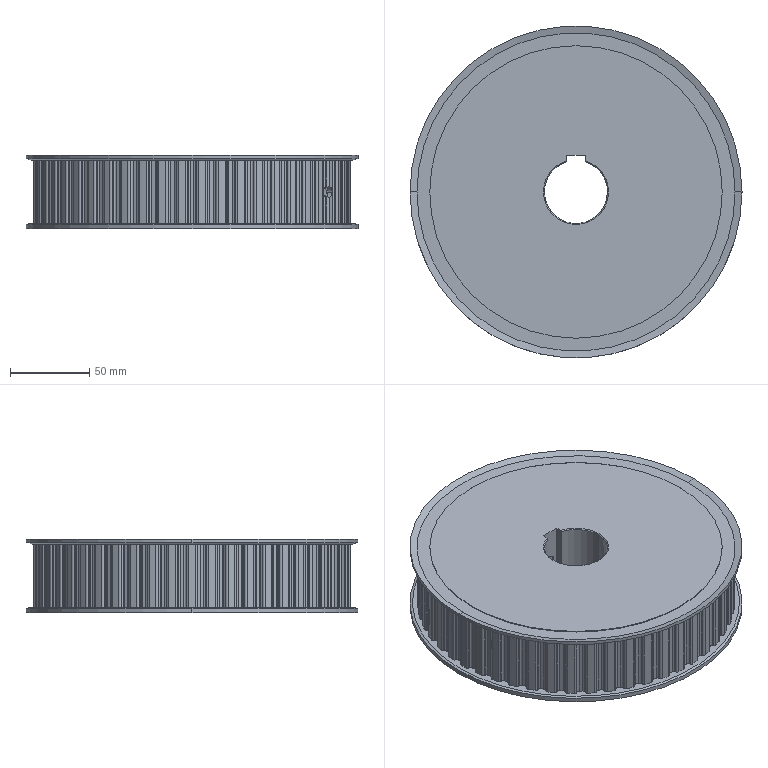Part | SolidWorks | features Revolution 6, ICE 4, RevCut 3, LockFeature 1 | 1 solid | 511 faces | box 210 x 210 x 46.349 mm | volume 1347722 mm3 | cylinder 367 | plane 130 | cone 14 | commonest cylinder face diameters 2.94 x123 2.84 x121 195.58 x51 200.76 x51 6.647 x8 185 x4